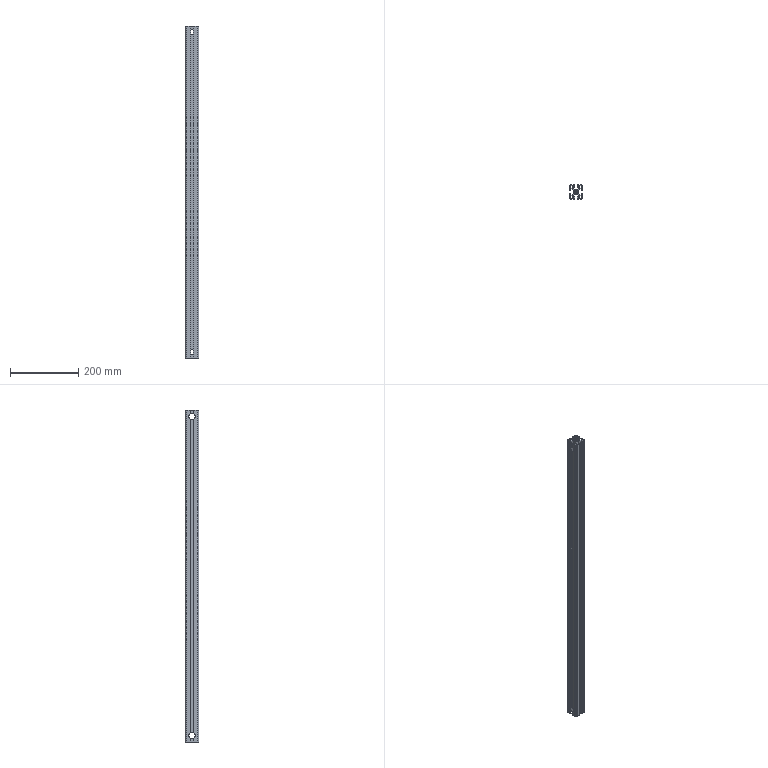Part | SolidWorks | features BaseBody 1, HoleWzd 1, MoveFace 1 | 1 solid | 235 faces | box 40 x 40 x 975 mm | volume 416243 mm3 | plane 166 | cylinder 69 | commonest cylinder face diameters 1.5 x18 2 x16 6.8 x15 19 x12 6.6 x4 9 x4